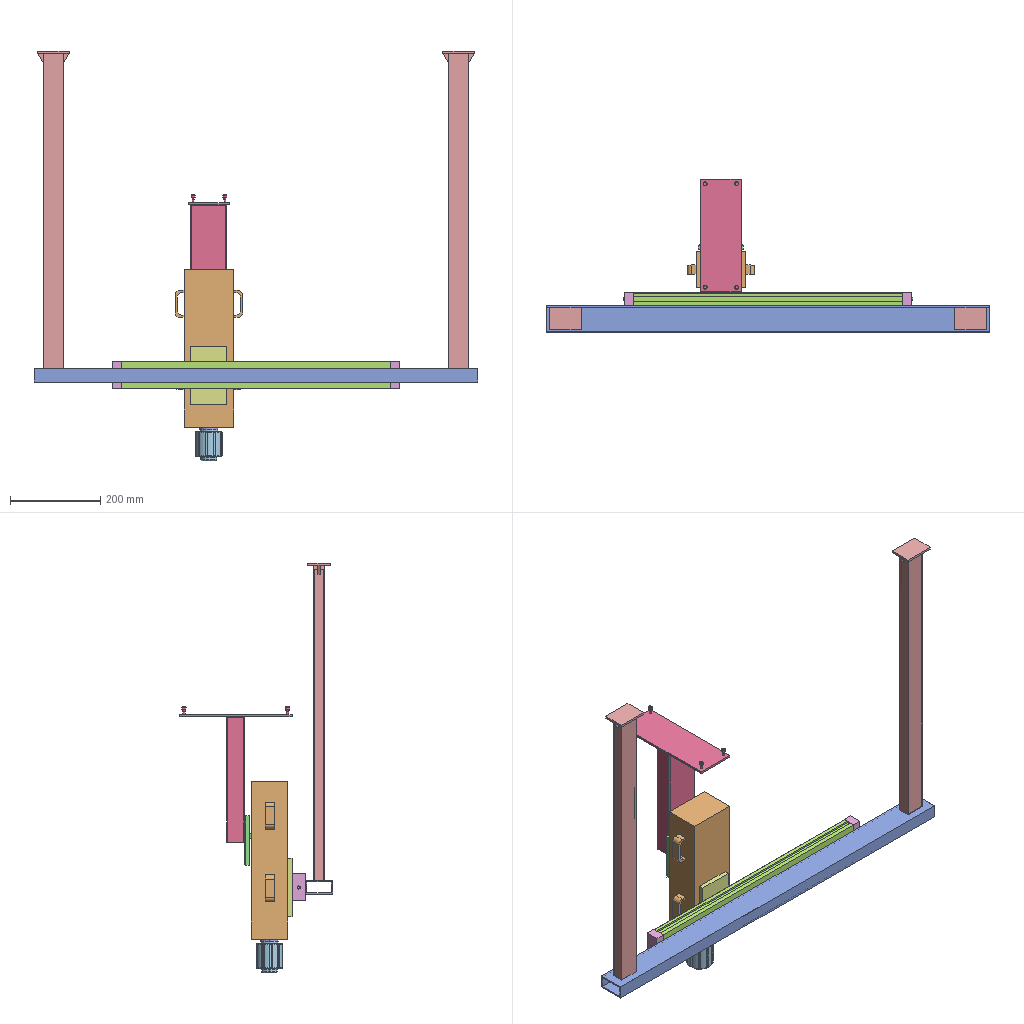Assembly | SolidWorks | 11 different items | 14 placed | box 986 x 340 x 910 mm
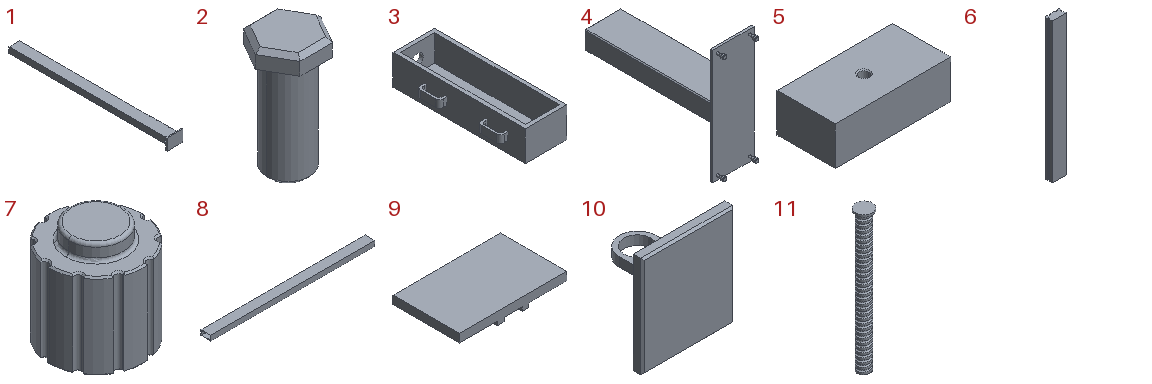Parts list (item | quantity | size | volume | features):
1 | x2 | 70 x 705 x 50 mm | 217416 mm3 | features ICE 3, Extrusion 1
2 | x2 | 7.616 x 6.595 x 14 mm | 306.418 mm3 | features Chamfer 1, Extrusion 1, ICE 1
3 | x1 | 150 x 350 x 80 mm | 1029931 mm3 | features Cut 2, Extrusion 1, Fillet 1, ICE 1, MirrorPattern 1, Shell 1
4 | x1 | 90 x 302 x 250 mm | 1008756 mm3 | features Chamfer 3, ICE 3, Extrusion 1, Fillet 1
5 | x2 | 60 x 30 x 20 mm | 35693 mm3 | features Extrusion 1, HoleWzd 1
6 | x1 | 60 x 30 x 598 mm | 978328 mm3 | features Chamfer 1, Cut 1, Extrusion 1
7 | x1 | 60 x 60 x 70 mm | 165967 mm3 | features ICE 2, Chamfer 1, Cut 1, Extrusion 1, Fillet 1
8 | x1 | 986 x 60 x 30 mm | 496944 mm3 | features Cut 1, Extrusion 1
9 | x1 | 130 x 80 x 15 mm | 110400 mm3 | features Extrusion 1, ICE 1
10 | x1 | 100 x 75 x 110 mm | 126385 mm3 | features Chamfer 1, Extrusion 1, ICE 1
11 | x1 | 40 x 40 x 335 mm | 211445 mm3 | features Extrusion 1, Helix 1, ICE 1, SweepCut 1
Mates (type | each side: item.copy, entity, surface, feature):
InPlace | 1.1 plane | assembly plane
InPlace | 1.2 face plane Boss-Extrude2 | 8.1 plane
InPlace | 6.1 plane | assembly plane
InPlace | 6.1 face plane Boss-Extrude1 | 5.1 plane
Coincident | 6.1 face plane Boss-Extrude1 | 5.2 face plane Boss-Extrude1
Coincident | 5.1 face plane Boss-Extrude1 | 5.2 face plane Boss-Extrude1 | 2 times
InPlace | 5.2 face plane Boss-Extrude1 | 2.1 plane
Concentric | 5.1 face cylinder M6 Tapped Hole1 | 2.2 face cylinder Boss-Extrude1
Coincident | 5.1 face plane Boss-Extrude1 | 2.2 face plane Boss-Extrude2
DistanceDim | 8.1 face plane Boss-Extrude1 | 3.1 face plane Boss-Extrude1
InPlace | 3.1 face plane Boss-Extrude1 | 11.1 plane
Concentric | 11.1 face cylinder Boss-Extrude1 | 10.1 face cylinder Boss-Extrude1
Parallel | 3.1 face plane Shell1 | 10.1 face plane Boss-Extrude2
InPlace | 10.1 face plane Boss-Extrude2 | 4.1 plane
InPlace | 11.1 face plane Boss-Extrude2 | 7.1 plane
Coincident | 6.1 face plane Cut-Extrude1 | 9.1 face plane Boss-Extrude2 | 2 times
Coincident | 3.1 face plane Boss-Extrude1 | 9.1 face plane Boss-Extrude1
Width | 3.1 face plane Boss-Extrude1 | 3.1 face plane Boss-Extrude1 | 9.1 face plane Boss-Extrude1 | 9.1 face plane Boss-Extrude1